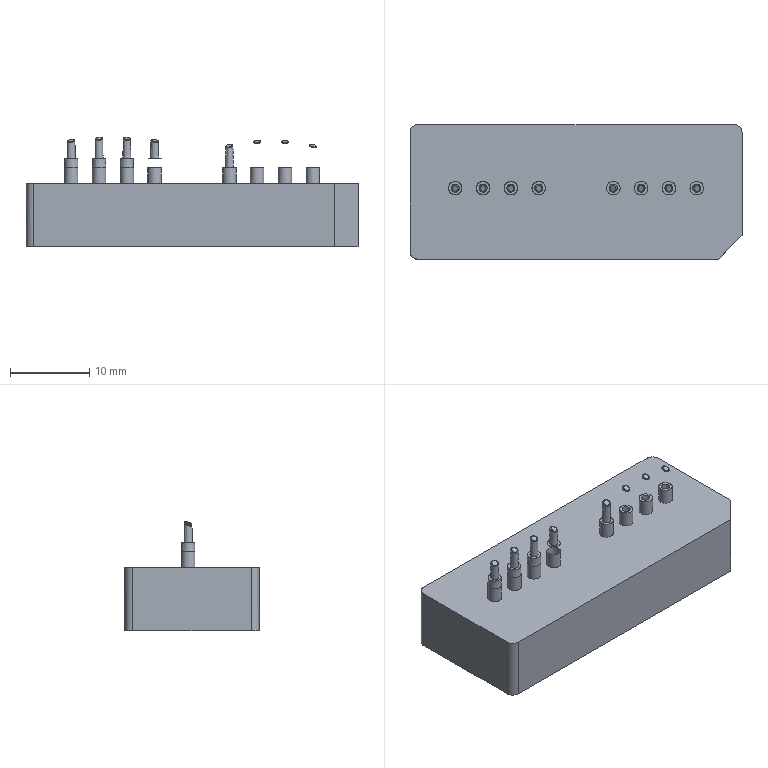NC program | PowerMill | posted by the shop | part box 42 x 17 x 13.856 mm
Lines 4063 to 5561 of 273708:
( TOOL ID   D3C_1_1 )
( TOOL DIA. 3. TIP RAD 0 LENGTH 61.04 )
( Z = -5.95 )
T15 M6
T26
G91 G28 Z0
G0 G90 G54
M08
S18000 M3
X0 Y0 M8
G43 Z9.805 H15
X-10.69 Y-1.921
Z.86
G1 Z-.34 F3000
X-10.681 Y-1.904 F5000
G3 X-10.753 Y-1.67 I-.153 J.081
G1 X-11.82 Y-1.108
X-12.242 Y-1.099
X-12.508 Y-1.055
X-12.664 Y-1.003
X-13.086 Y-.759
X-13.231 Y-.633
X-13.508 Y-.262
X-13.671 Y.211
X-13.709 Y.633
X-13.642 Y1.055
X-13.508 Y1.391
X-13.139 Y1.9
X-12.664 Y2.236
X-12.486 Y2.322
X-12.242 Y2.399
X-11.82 Y2.458
X-11.398 Y2.424
X-11.032 Y2.322
X-10.553 Y2.053
X-10.376 Y1.9
X-10.131 Y1.6
G3 X-9.874 Y1.579 I.135 J.066
G1 X-9.709 Y1.809
X-9.287 Y2.163
X-8.966 Y2.322
X-8.443 Y2.442
X-8.021 Y2.441
X-7.598 Y2.352
X-7.176 Y2.148
X-6.859 Y1.9
X-6.536 Y1.477
X-6.36 Y1.055
X-6.289 Y.633
X-6.328 Y.211
X-6.468 Y-.211
X-6.754 Y-.617
X-7.176 Y-.931
X-7.492 Y-1.055
X-8.021 Y-1.105
X-8.865 Y-1.092
X-9.032 Y-1.055
X-9.287 Y-.951
X-9.725 Y-.633
X-9.87 Y-.434
G3 X-10.04 Y-.384 I-.117 J-.082
G1 X-10.066 Y-.393
X-10.107 Y-.428
X-10.274 Y-.633
X-10.553 Y-.856
X-10.975 Y-1.055
X-11.398 Y-1.117
X-11.82 Y-1.108
X-10.965 Y-2.286 Z-.485
X-10.955 Y-2.27
G3 X-11.003 Y-2.03 I-.144 J.096
G1 X-11.863 Y-1.459
X-12.242 Y-1.412
X-12.664 Y-1.261
X-13.086 Y-.986
X-13.398 Y-.633
X-13.508 Y-.457
X-13.536 Y-.389
X-13.575 Y-.326
G3 X-13.8 Y-.332 I-.11 J-.102
G1 X-13.93 Y-.487
X-14.117 Y-.633
X-14.353 Y-.76
X-14.775 Y-.872
X-15.197 Y-.859
X-15.619 Y-.734
X-16.041 Y-.552
X-16.463 Y-.243
X-16.778 Y.211
X-16.885 Y.602
X-16.886 Y1.055
X-16.763 Y1.477
X-16.463 Y1.905
X-16.041 Y2.224
X-15.822 Y2.322
X-15.619 Y2.381
X-15.197 Y2.418
X-14.775 Y2.358
X-14.353 Y2.194
X-13.951 Y1.9
X-13.67 Y1.531
G3 X-13.432 Y1.531 I.119 J.091
G1 X-13.146 Y1.9
X-12.664 Y2.245
X-12.455 Y2.329
X-12.242 Y2.404
X-11.82 Y2.459
X-11.398 Y2.427
X-11.022 Y2.322
X-10.553 Y2.054
X-10.372 Y1.9
X-10.306 Y1.815
X-10.131 Y1.6
G3 X-9.874 Y1.579 I.135 J.066
G1 X-9.827 Y1.644
X-9.709 Y1.813
X-9.287 Y2.164
X-9.078 Y2.267
X-8.865 Y2.362
X-8.443 Y2.445
X-8.021
X-7.598 Y2.356
X-7.176 Y2.151
X-6.855 Y1.9
X-6.569 Y1.532
G3 X-6.332 Y1.532 I.118 J.092
G1 X-6.043 Y1.9
X-5.91 Y2.018
X-5.488 Y2.271
X-5.066 Y2.39
X-4.643 Y2.417
X-4.221 Y2.334
X-3.799 Y2.128
X-3.522 Y1.9
X-3.377 Y1.721
X-3.238 Y1.477
X-3.119 Y1.055
X-3.126 Y.633
X-3.235 Y.211
X-3.377 Y-.049
X-3.506 Y-.211
X-3.799 Y-.461
X-4.221 Y-.666
X-4.643 Y-.829
X-5.066 Y-.875
X-5.488 Y-.807
X-5.852 Y-.633
X-6.207 Y-.285
G3 X-6.446 Y-.325 I-.105 J-.107
G1 X-6.601 Y-.633
X-6.754 Y-.823
X-7.001 Y-1.055
X-7.176 Y-1.175
X-7.598 Y-1.369
X-8.021 Y-1.454
X-8.443 Y-1.456
X-8.865 Y-1.378
X-9.287 Y-1.185
X-9.486 Y-1.055
X-9.709 Y-.844
X-9.883 Y-.633
G3 X-10.121 Y-.636 I-.118 J-.09
G1 X-10.126 Y-.643
X-10.131 Y-.65
X-10.516 Y-1.055
X-10.975 Y-1.322
X-11.398 Y-1.437
X-11.82 Y-1.464
X-11.863 Y-1.459
X-10.917 Y-2.32 Z-.63
X-10.907 Y-2.304
G3 X-10.962 Y-2.065 I-.147 J.092
G1 X-11.867 Y-1.501
X-12.117 Y-1.477
X-12.664 Y-1.293
X-13.02 Y-1.055
X-13.081 Y-.989
X-13.086 Y-.986
X-13.138 Y-.926
X-13.409 Y-.633
X-13.415 Y-.623
X-13.423 Y-.613
G3 X-13.669 Y-.614 I-.123 J-.082
G1 X-13.682 Y-.633
X-13.93 Y-.885
X-14.182 Y-1.055
X-14.353 Y-1.14
X-14.775 Y-1.252
X-15.197 Y-1.245
X-15.619 Y-1.116
X-16.463 Y-.74
X-16.606 Y-.633
X-16.885 Y-.341
X-16.968 Y-.211
X-17.142 Y.211
X-17.198 Y.633
X-17.139 Y1.055
X-16.971 Y1.477
X-16.885 Y1.626
X-16.661 Y1.9
X-16.463 Y2.07
X-16.041 Y2.313
X-15.619 Y2.43
X-15.197 Y2.462
X-14.775 Y2.4
X-14.353 Y2.237
X-13.93 Y1.94
X-13.638 Y1.559
X-13.62 Y1.544
G3 X-13.406 Y1.563 I.098 J.11
G1 X-13.215 Y1.81
X-13.149 Y1.9
X-12.664 Y2.246
X-12.454 Y2.33
X-12.242 Y2.407
X-11.82 Y2.46
X-11.398 Y2.43
X-11.016 Y2.322
X-10.553 Y2.057
X-10.369 Y1.9
X-10.26 Y1.757
X-10.131 Y1.6
G3 X-9.886 Y1.567 I.134 J.064
G1 X-9.876 Y1.577
X-9.867 Y1.589
X-9.709 Y1.817
X-9.287 Y2.166
X-9.168 Y2.222
X-8.966 Y2.322
X-8.947 Y2.326
X-8.865 Y2.365
X-8.443 Y2.449
X-8.021 Y2.45
X-7.598 Y2.359
X-7.176 Y2.153
X-6.851 Y1.9
X-6.754 Y1.797
X-6.613 Y1.59
G3 X-6.362 Y1.594 I.124 J.085
G1 X-6.332 Y1.642
X-6.111 Y1.9
X-5.91 Y2.071
X-5.467 Y2.322
X-5.066 Y2.432
X-4.643 Y2.46
X-4.221 Y2.399
X-3.981 Y2.322
X-3.799 Y2.232
X-3.377 Y1.933
X-3.024 Y1.477
X-2.857 Y1.055
X-2.806 Y.633
X-2.854 Y.211
X-3.032 Y-.211
X-3.377 Y-.623
X-3.799 Y-.874
X-4.643 Y-1.213
X-5.066 Y-1.261
X-5.488 Y-1.194
X-5.91 Y-1.003
X-6.332 Y-.605
G3 X-6.539 Y-.561 I-.126 J-.082
G1 X-6.569 Y-.589
X-6.586 Y-.608
X-6.599 Y-.63
X-6.601 Y-.633
X-6.628 Y-.667
X-6.754 Y-.843
X-6.978 Y-1.055
X-7.176 Y-1.201
X-7.598 Y-1.402
X-7.879 Y-1.477
X-8.021 Y-1.497
X-8.443 Y-1.493
X-8.865 Y-1.408
X-9.287 Y-1.212
X-9.505 Y-1.055
X-9.709 Y-.862
X-9.882 Y-.644
G3 X-10.131 Y-.666 I-.118 J-.093
G1 X-10.495 Y-1.055
X-10.975 Y-1.351
X-11.398 Y-1.477
X-11.82 Y-1.505
X-11.867 Y-1.501
X-10.955 Y-2.332 Z-.774
X-10.944 Y-2.315
G3 X-10.995 Y-2.076 I-.145 J.095
G1 X-11.868 Y-1.507
X-12.126 Y-1.477
X-12.664 Y-1.296
X-13.025 Y-1.055
X-13.408 Y-.638
G3 X-13.632 Y-.641 I-.111 J-.101
G1 X-13.93 Y-.99
X-14.353 Y-1.281
X-14.775 Y-1.433
X-15.197 Y-1.483
X-15.619 Y-1.443
X-16.041 Y-1.31
X-16.463 Y-1.072
X-16.9 Y-.633
X-17.133 Y-.211
X-17.241 Y.211
X-17.254 Y.633
X-17.179 Y1.055
X-16.991 Y1.477
X-16.885 Y1.648
X-16.667 Y1.9
X-16.463 Y2.072
X-16.041 Y2.315
X-15.619 Y2.434
X-15.197 Y2.465
X-14.775 Y2.401
X-14.525 Y2.322
X-14.353 Y2.24
X-13.93 Y1.941
X-13.639 Y1.562
X-13.623 Y1.547
G3 X-13.406 Y1.564 I.101 J.107
G1 X-13.283 Y1.722
X-13.152 Y1.9
X-12.664 Y2.248
X-12.574 Y2.281
X-12.486 Y2.322
X-12.363 Y2.362
X-12.242 Y2.409
X-11.82 Y2.46
X-11.398 Y2.434
X-11.011 Y2.322
X-10.553 Y2.06
X-10.365 Y1.9
X-10.226 Y1.716
X-10.131 Y1.6
X-10.125 Y1.59
X-10.111 Y1.573
G3 X-9.889 Y1.566 I.114 J.093
G1 X-9.876 Y1.58
X-9.709 Y1.821
X-9.287 Y2.167
X-9.08 Y2.265
X-8.966 Y2.322
X-8.954 Y2.325
X-8.943 Y2.33
X-8.865 Y2.367
X-8.443 Y2.452
X-8.021
X-7.598 Y2.362
X-7.176 Y2.154
X-6.848 Y1.9
X-6.754 Y1.801
X-6.614 Y1.595
G3 X-6.362 Y1.601 I.124 J.085
G1 X-6.332 Y1.65
X-6.113 Y1.9
X-5.91 Y2.073
X-5.474 Y2.322
X-5.066 Y2.434
X-4.643 Y2.466
X-4.221 Y2.401
X-4.007 Y2.329
X-3.799 Y2.241
X-3.377 Y1.942
X-3.005 Y1.477
X-2.82 Y1.055
X-2.743 Y.633
X-2.755 Y.211
X-2.87 Y-.211
X-2.955 Y-.4
X-3.099 Y-.633
X-3.377 Y-.944
X-3.799 Y-1.228
X-4.221 Y-1.398
X-4.656 Y-1.477
X-5.066 Y-1.464
X-5.488 Y-1.346
X-5.91 Y-1.116
X-6.332 Y-.696
X-6.378 Y-.629
X-6.447 Y-.586
X-6.502 Y-.581
X-6.555 Y-.596
X-6.583 Y-.618
X-6.596 Y-.629
X-6.608 Y-.642
X-6.616 Y-.652
X-6.754 Y-.846
X-6.975 Y-1.055
X-7.176 Y-1.204
X-7.598 Y-1.406
X-7.808 Y-1.459
X-8.021 Y-1.499
X-8.443
X-8.865 Y-1.411
X-9.287 Y-1.215
X-9.507 Y-1.055
X-9.709 Y-.865
X-9.882 Y-.648
G3 X-10.122 Y-.657 I-.117 J-.091
G1 X-10.127 Y-.663
X-10.131 Y-.67
X-10.495 Y-1.055
X-10.975 Y-1.353
X-11.398 Y-1.477
X-11.82 Y-1.513
X-11.868 Y-1.507
X-10.969 Y-2.336 Z-.919
X-10.958 Y-2.32
G3 X-11.007 Y-2.08 I-.144 J.096
G1 X-11.868 Y-1.51
X-12.131 Y-1.477
X-12.664 Y-1.299
X-13.028 Y-1.055
X-13.407 Y-.641
G3 X-13.631 Y-.644 I-.111 J-.101
G1 X-13.93 Y-.99
X-14.353 Y-1.289
X-14.775 Y-1.45
X-15.197 Y-1.514
X-15.665 Y-1.477
X-16.041 Y-1.362
X-16.463 Y-1.124
X-16.885 Y-.698
X-17.146 Y-.211
X-17.244 Y.211
X-17.258 Y.633
X-17.18 Y1.055
X-16.995 Y1.477
X-16.885 Y1.655
X-16.667 Y1.9
X-16.463 Y2.074
X-16.041 Y2.317
X-15.619 Y2.438
X-15.197 Y2.468
X-14.775 Y2.402
X-14.519 Y2.322
X-14.353 Y2.243
X-13.93 Y1.943
X-13.64 Y1.565
X-13.594 Y1.525
X-13.535 Y1.509
X-13.463 Y1.52
X-13.405 Y1.565
X-13.346 Y1.641
X-13.156 Y1.9
X-12.664 Y2.25
X-12.519 Y2.306
X-12.486 Y2.322
X-12.438 Y2.337
X-12.242 Y2.412
X-11.82 Y2.461
X-11.398 Y2.437
X-11.005 Y2.322
X-10.553 Y2.063
X-10.362 Y1.9
X-10.131 Y1.613
G3 X-9.871 Y1.591 I.136 J.066
G1 X-9.709 Y1.824
X-9.287 Y2.168
X-8.865 Y2.37
X-8.443 Y2.454
X-8.021 Y2.455
X-7.598 Y2.364
X-7.176 Y2.155
X-6.844 Y1.9
X-6.754 Y1.804
X-6.613 Y1.599
G3 X-6.361 Y1.606 I.124 J.085
G1 X-6.332 Y1.654
X-6.116 Y1.9
X-5.91 Y2.074
X-5.488 Y2.319
X-5.066 Y2.435
X-4.643 Y2.47
X-4.221 Y2.403
X-4.009 Y2.328
X-3.799 Y2.244
X-3.377 Y1.944
X-3.002 Y1.477
X-2.819 Y1.055
X-2.737 Y.633
X-2.753 Y.211
X-2.856 Y-.211
X-3.07 Y-.633
X-3.377 Y-.988
X-3.799 Y-1.285
X-4.337 Y-1.477
X-4.643 Y-1.514
X-5.066 Y-1.485
X-5.488 Y-1.364
X-5.696 Y-1.235
X-5.91 Y-1.116
X-5.949 Y-1.081
X-5.995 Y-1.055
X-6.332 Y-.701
X-6.373 Y-.638
X-6.434 Y-.594
G3 X-6.609 Y-.647 I-.053 J-.14
G1 X-6.754 Y-.849
X-6.973 Y-1.055
X-7.176 Y-1.207
X-7.598 Y-1.409
X-7.809 Y-1.458
X-8.021 Y-1.501
X-8.443 Y-1.503
X-8.865 Y-1.413
X-9.287 Y-1.218
X-9.509 Y-1.055
X-9.709 Y-.868
X-9.882 Y-.652
G3 X-10.131 Y-.674 I-.117 J-.094
G1 X-10.494 Y-1.055
X-10.975 Y-1.356
X-11.398 Y-1.477
X-11.82 Y-1.515
X-11.868 Y-1.51
X-10.98 Y-2.341 Z-1.064
X-10.969 Y-2.325
G3 X-11.017 Y-2.084 I-.144 J.097
G1 X-11.868 Y-1.512
X-12.136 Y-1.477
X-12.664 Y-1.302
X-13.03 Y-1.055
X-13.408 Y-.644
G3 X-13.631 Y-.647 I-.11 J-.101
G1 X-13.93 Y-.99
X-14.353 Y-1.292
X-14.775 Y-1.45
X-15.197 Y-1.517
X-15.619 Y-1.487
X-15.65 Y-1.479
X-15.665 Y-1.477
X-15.812 Y-1.432
X-16.041 Y-1.367
X-16.463 Y-1.126
X-16.885 Y-.7
X-17.148 Y-.211
X-17.248 Y.211
X-17.262 Y.633
X-17.183 Y1.055
X-17. Y1.477
X-16.885 Y1.66
X-16.667 Y1.9
X-16.463 Y2.076
X-16.041 Y2.32
X-15.619 Y2.44
X-15.197 Y2.471
X-14.775 Y2.403
X-14.512 Y2.322
X-14.353 Y2.246
X-13.93 Y1.946
X-13.642 Y1.568
G3 X-13.402 Y1.571 I.119 J.091
G1 X-13.159 Y1.9
X-12.664 Y2.252
X-12.496 Y2.317
X-12.486 Y2.322
X-12.473 Y2.326
X-12.242 Y2.415
X-11.82 Y2.462
X-11.398 Y2.44
X-10.999 Y2.322
X-10.553 Y2.067
X-10.358 Y1.9
X-10.131 Y1.617
G3 X-9.872 Y1.596 I.136 J.066
G1 X-9.709 Y1.828
X-9.287 Y2.169
X-8.865 Y2.373
X-8.443 Y2.457
X-8.021
X-7.598 Y2.367
X-7.176 Y2.158
X-6.841 Y1.9
X-6.754 Y1.808
X-6.613 Y1.603
G3 X-6.361 Y1.611 I.124 J.085
G1 X-6.332 Y1.659
X-6.12 Y1.9
X-5.91 Y2.076
X-5.488 Y2.322
X-5.066 Y2.437
X-4.643 Y2.472
X-4.221 Y2.405
X-4.113 Y2.364
X-3.981 Y2.322
X-3.892 Y2.28
X-3.799 Y2.247
X-3.377 Y1.946
X-2.999 Y1.477
X-2.816 Y1.055
X-2.734 Y.633
X-2.75 Y.211
X-2.851 Y-.211
X-3.07 Y-.633
X-3.377 Y-.993
X-3.799 Y-1.289
X-4.334 Y-1.477
X-4.643 Y-1.517
X-5.066 Y-1.485
X-5.488 Y-1.367
X-5.804 Y-1.174
X-5.91 Y-1.116
X-5.928 Y-1.098
X-5.998 Y-1.055
X-6.332 Y-.705
X-6.373 Y-.642
X-6.433 Y-.598
X-6.518 Y-.591
X-6.592 Y-.633
X-6.609 Y-.651
X-6.754 Y-.852
X-6.97 Y-1.055
X-7.176 Y-1.21
X-7.598 Y-1.411
X-7.788 Y-1.453
X-7.858 Y-1.473
X-7.93 Y-1.484
X-8.021 Y-1.504
X-8.443 Y-1.506
X-8.865 Y-1.416
X-9.287 Y-1.222
X-9.511 Y-1.055
X-9.709 Y-.872
X-9.882 Y-.656
G3 X-10.131 Y-.679 I-.117 J-.094
G1 X-10.491 Y-1.055
X-10.975 Y-1.359
X-11.398 Y-1.477
X-11.82 Y-1.518
X-11.868 Y-1.512
X-10.989 Y-2.345 Z-1.209
X-10.978 Y-2.329
G3 X-11.024 Y-2.088 I-.143 J.097
G1 X-11.869 Y-1.514
X-12.141 Y-1.477
X-12.664 Y-1.305
X-13.032 Y-1.055
X-13.408 Y-.647
G3 X-13.631 Y-.65 I-.11 J-.102
G1 X-13.93 Y-.99
X-14.353 Y-1.295
X-14.775 Y-1.451
X-15.197 Y-1.519
X-15.619 Y-1.491
X-16.041 Y-1.369
X-16.463 Y-1.128
X-16.885 Y-.704
X-17.151 Y-.211
X-17.251 Y.211
X-17.265 Y.633
X-17.186 Y1.055
X-17.003 Y1.477
X-16.885 Y1.664
X-16.669 Y1.9
X-16.463 Y2.078
X-16.041 Y2.322
X-15.619 Y2.442
X-15.197 Y2.473
X-14.775 Y2.405
X-14.506 Y2.322
X-14.353 Y2.249
X-13.93 Y1.949
X-13.635 Y1.577
G3 X-13.397 Y1.582 I.117 J.093
G1 X-13.163 Y1.9
X-12.664 Y2.254
X-12.242 Y2.417
X-11.82 Y2.463
X-11.398 Y2.442
X-11.068 Y2.342
X-10.999 Y2.322
X-10.993 Y2.32
X-10.987 Y2.318
X-10.975 Y2.314
X-10.553 Y2.069
X-10.355 Y1.9
X-10.131 Y1.62
G3 X-9.872 Y1.599 I.136 J.067
G1 X-9.709 Y1.832
X-9.287 Y2.17
X-8.865 Y2.375
X-8.443 Y2.459
X-8.021 Y2.46
X-7.598 Y2.369
X-7.176 Y2.161
X-6.837 Y1.9
X-6.826 Y1.884
X-6.754 Y1.808
X-6.613 Y1.603
X-6.549 Y1.551
X-6.467 Y1.54
X-6.44 Y1.549
X-6.404 Y1.569
X-6.374 Y1.598
X-6.365 Y1.608
X-6.332 Y1.663
X-6.124 Y1.9
X-5.91 Y2.077
X-5.494 Y2.322
X-5.066 Y2.439
X-4.643 Y2.475
X-4.221 Y2.406
X-4.072 Y2.351
X-4.007 Y2.332
X-3.945 Y2.304
X-3.799 Y2.25
X-3.377 Y1.948
X-2.996 Y1.477
X-2.813 Y1.055
X-2.732 Y.633
X-2.748 Y.211
X-2.848 Y-.211
X-3.067 Y-.633
X-3.377 Y-.996
X-3.799 Y-1.293
X-4.332 Y-1.477
X-4.643 Y-1.519
X-5.066 Y-1.485
X-5.488 Y-1.37
X-5.832 Y-1.158
X-5.91 Y-1.116
X-5.924 Y-1.102
X-6. Y-1.055
X-6.332 Y-.709
X-6.373 Y-.645
X-6.434 Y-.6
G3 X-6.611 Y-.653 I-.054 J-.14
G1 X-6.754 Y-.855
X-6.787 Y-.883
X-6.97 Y-1.055
X-7.146 Y-1.187
X-7.176 Y-1.213
X-7.598 Y-1.413
X-7.834 Y-1.465
X-7.879 Y-1.477
X-7.903 Y-1.481
X-8.021 Y-1.507
X-8.443 Y-1.508
X-8.865 Y-1.418
X-9.287 Y-1.224
X-9.32 Y-1.197
X-9.511 Y-1.055
X-9.678 Y-.901
X-9.709 Y-.875
X-9.882 Y-.66
G3 X-10.131 Y-.683 I-.117 J-.094
G1 X-10.489 Y-1.055
X-10.975 Y-1.361
X-11.395 Y-1.477
X-11.82 Y-1.521
X-11.869 Y-1.514
G0 Z3.57
G1 X5.805 Y-.192 F10000
G0 Z.57
G1 Z-.63 F3000
X5.822 Y-.202 F5000
G3 X6.058 Y-.137 I.086 J.151
G1 X6.496 Y.633
X6.519 Y1.055
X6.667 Y1.477
X6.754 Y1.625
X6.983 Y1.9
X7.176 Y2.068
X7.598 Y2.305
X8.021 Y2.408
X8.443 Y2.409
X8.865 Y2.317
X9.287 Y2.108
X9.542 Y1.9
X9.709 Y1.713
X9.858 Y1.477
X9.863 Y1.468
X9.868 Y1.458
G3 X10.141 Y1.477 I.132 J.069
G1 X10.463 Y1.9
X10.553 Y1.985
X10.975 Y2.257
X11.135 Y2.322
X11.398 Y2.383
X11.82 Y2.423
X12.242 Y2.357
X12.664 Y2.172
X13.017 Y1.9
X13.335 Y1.477
X13.483 Y1.055
X13.504 Y.633
X13.401 Y.211
X13.158 Y-.211
X13.086 Y-.296
X12.64 Y-.633
X12.242 Y-.763
X11.82 Y-.832
X11.398 Y-.864
X10.975 Y-.778
X10.674 Y-.633
X10.553 Y-.548
X10.219 Y-.211
X10.131 Y-.074
G3 X9.858 Y-.061 I-.139 J-.056
G1 X9.781 Y-.211
X9.709 Y-.304
X9.327 Y-.633
X8.865 Y-.828
X8.443 Y-.865
X7.598 Y-.724
X7.364 Y-.633
X7.176 Y-.522
X6.842 Y-.211
X6.596 Y.211
X6.496 Y.633
X5.482 Y-.17 Z-.774
X5.498 Y-.181
G3 X5.739 Y-.14 I.1 J.141
G1 X6.309 Y.662
X6.37 Y1.055
X6.546 Y1.477
X6.754 Y1.765
X6.88 Y1.9
X7.176 Y2.133
X7.549 Y2.322
X8.021 Y2.435
X8.443 Y2.431
X8.865 Y2.341
X9.287 Y2.145
X9.605 Y1.9
X9.709 Y1.789
X9.867 Y1.559
G3 X10.12 Y1.568 I.124 J.085
G1 X10.131 Y1.587
X10.396 Y1.9
X10.553 Y2.034
X10.975 Y2.285
X11.398 Y2.411
X11.82 Y2.441
X12.242 Y2.384
X12.452 Y2.322
X12.664 Y2.223
X13.086 Y1.932
X13.453 Y1.477
X13.631 Y1.055
X13.695 Y.633
X13.667 Y.211
X13.508 Y-.226
X13.208 Y-.633
X13.086 Y-.746
X12.664 Y-.996
X12.473 Y-1.055
X12.242 Y-1.098
X11.398 Y-1.206
X10.975 Y-1.134
X10.779 Y-1.055
X10.553 Y-.925
X10.217 Y-.633
X10.121 Y-.493
G3 X9.869 Y-.498 I-.124 J-.085
G1 X9.709 Y-.717
X9.287 Y-1.02
X8.865 Y-1.174
X8.443 Y-1.2
X7.523 Y-1.055
X7.176 Y-.921
X6.786 Y-.633
X6.478 Y-.211
X6.333 Y.211
X6.304 Y.633
X6.309 Y.662
X5.405 Y-.206 Z-.919
X5.421 Y-.217
G3 X5.663 Y-.179 I.102 J.14
G1 X6.281 Y.667
X6.332 Y.968
X6.541 Y1.477
X6.596 Y1.547
X6.754 Y1.765
X6.85 Y1.867
X6.854 Y1.872
X6.875 Y1.9
X7.176 Y2.137
X7.543 Y2.322
X8.021 Y2.438
X8.443 Y2.432
X8.865 Y2.346
X9.287 Y2.149
X9.608 Y1.9
X9.709 Y1.795
X9.867 Y1.561
G3 X10.121 Y1.569 I.124 J.084
G1 X10.131 Y1.587
X10.392 Y1.9
X10.553 Y2.036
X10.975 Y2.288
X11.398 Y2.413
X11.82 Y2.445
X12.242 Y2.387
X12.457 Y2.322
X12.664 Y2.226
X13.086 Y1.937
X13.458 Y1.477
X13.643 Y1.055
X13.725 Y.633
X13.711 Y.211
X13.606 Y-.211
X13.508 Y-.426
X13.376 Y-.633
X13.086 Y-.958
X12.97 Y-1.055
X12.664 Y-1.244
X12.242 Y-1.393
X11.82 Y-1.457
X11.398 Y-1.436
X10.975 Y-1.314
X10.553 Y-1.071
X10.129 Y-.633
G3 X9.872 Y-.61 I-.136 J-.065
G1 X9.709 Y-.834
X9.47 Y-1.055
X9.287 Y-1.181
X8.865 Y-1.372
X8.443 Y-1.453
X8.021 Y-1.441
X7.598 Y-1.348
X7.176 Y-1.157
X7.029 Y-1.055
X6.754 Y-.804
X6.62 Y-.633
X6.398 Y-.211
X6.287 Y.211
X6.275 Y.633
X6.281 Y.667
X4.64 Y3.219 Z-1.064
X4.636 Y3.201
G3 X4.766 Y2.993 I.169 J-.038
G1 X7.631 Y2.345
X8.021 Y2.44
X8.443 Y2.433
X8.865 Y2.352
X9.287 Y2.152
X9.33 Y2.116
X9.608 Y1.9
X9.686 Y1.819
X9.709 Y1.8
X9.867 Y1.564
G3 X10.131 Y1.589 I.125 J.085
G1 X10.388 Y1.9
X10.553 Y2.039
X10.975 Y2.291
X11.398 Y2.415
X11.82 Y2.448
X12.242 Y2.39
X12.463 Y2.322
X12.664 Y2.227
X13.086 Y1.94
X13.454 Y1.486
G3 X13.689 Y1.488 I.117 J.094
G1 X14.01 Y1.9
X14.353 Y2.143
X14.775 Y2.315
X15.197 Y2.379
X15.619 Y2.324
X16.041 Y2.147
X16.354 Y1.9
X16.463 Y1.775
X16.64 Y1.477
X16.766 Y1.055
X16.761 Y.633
X16.635 Y.211
X16.463 Y-.091
X16.363 Y-.211
X16.041 Y-.488
X15.619 Y-.697
X15.197 Y-.803
X14.775 Y-.787
X14.353 Y-.664
X13.93 Y-.366
X13.816 Y-.243
X13.795 Y-.227
G3 X13.573 Y-.284 I-.089 J-.117
G1 X13.544 Y-.346
X13.508 Y-.438
X13.391 Y-.633
X13.086 Y-.982
X12.664 Y-1.271
X12.242 Y-1.436
X12.041 Y-1.477
X11.82 Y-1.493
X11.491 Y-1.477
X10.975 Y-1.334
X10.553 Y-1.083
X10.344 Y-.855
X10.129 Y-.633
G3 X9.89 Y-.614 I-.126 J-.075
G1 X9.882 Y-.624
X9.878 Y-.628
X9.875 Y-.633
X9.709 Y-.839
X9.486 Y-1.055
X9.287 Y-1.197
X8.865 Y-1.395
X8.515 Y-1.477
X7.958
X7.598 Y-1.387
X7.176 Y-1.186
X6.997 Y-1.055
X6.754 Y-.817
X6.611 Y-.633
X6.417 Y-.256
G3 X6.176 Y-.22 I-.133 J-.069
G1 X5.91 Y-.493
X5.68 Y-.633
X5.488 Y-.713
X5.066 Y-.796
X4.643 Y-.771
X4.245 Y-.633
X3.799 Y-.363
X3.645 Y-.211
X3.371 Y.211
X3.245 Y.633
X3.244 Y1.055
X3.364 Y1.477
X3.65 Y1.9
X3.799 Y2.026
X4.221 Y2.27
X4.395 Y2.322
X4.643 Y2.357
X5.066 Y2.346
X5.488 Y2.222
X5.91 Y1.955
X6.307 Y1.477
G3 X6.54 Y1.48 I.115 J.096
G1 X6.702 Y1.692
X6.871 Y1.9
X7.176 Y2.141
X7.538 Y2.322
X7.631 Y2.345
X4.616 Y3.346 Z-1.209
X4.611 Y3.327
G3 X4.743 Y3.12 I.169 J-.038
G1 X7.899 Y2.413
X8.021 Y2.443
X8.443 Y2.434
X8.865 Y2.355
X9.287 Y2.154
X9.502 Y1.984
X9.709 Y1.803
X9.866 Y1.567
G3 X10.121 Y1.575 I.125 J.083
G1 X10.131 Y1.593
X10.384 Y1.9
X10.553 Y2.04
X10.975 Y2.293
X11.398 Y2.417
X11.82 Y2.451
X12.242 Y2.393
X12.468 Y2.322
X12.664 Y2.23
X12.9 Y2.068
X13.132 Y1.9
X13.266 Y1.719
X13.407 Y1.544
G3 X13.621 Y1.528 I.114 J.093
G1 X13.638 Y1.544
X13.904 Y1.9
X14.353 Y2.223
X14.563 Y2.322
X14.775 Y2.388
X15.197 Y2.448
X15.619 Y2.425
X15.976 Y2.322
X16.463 Y2.039
X16.623 Y1.9
X16.885 Y1.55
X17.075 Y1.055
X17.112 Y.633
X17.029 Y.211
X16.811 Y-.211
X16.463 Y-.562
X15.498 Y-1.055
X15.197 Y-1.137
X14.775 Y-1.148
X14.353 Y-1.051
X13.93 Y-.805
X13.754 Y-.633
X13.69 Y-.544
G3 X13.438 Y-.557 I-.122 J-.087
G1 X13.394 Y-.633
X13.086 Y-.986
X12.664 Y-1.277
X12.242 Y-1.439
X12.058 Y-1.477
X11.82 Y-1.497
X11.491 Y-1.477
X10.975 Y-1.338
X10.553 Y-1.086
X10.295 Y-.804
X10.129 Y-.633
G3 X9.894 Y-.614 I-.125 J-.078
G1 X9.877 Y-.633
X9.709 Y-.843
X9.489 Y-1.055
X9.287 Y-1.199
X8.865 Y-1.397
X8.515 Y-1.477
X8.021 Y-1.485
X7.99 Y-1.478
X7.958 Y-1.477
X7.604 Y-1.388
X7.598 Y-1.387
X7.176 Y-1.189
X6.992 Y-1.055
X6.754 Y-.822
X6.607 Y-.633
X6.574 Y-.571
X6.53 Y-.515
G3 X6.31 Y-.54 I-.099 J-.113
G1 X6.243 Y-.633
X5.91 Y-.914
X5.488 Y-1.097
X5.066 Y-1.154
X4.643 Y-1.097
X4.519 Y-1.055
X3.653 Y-.633
X3.377 Y-.423
X3.196 Y-.211
X2.976 Y.211
X2.892 Y.633
X2.928 Y1.055
X3.08 Y1.477
X3.381 Y1.9
X3.799 Y2.215
X4.221 Y2.386
X4.643 Y2.452
X5.066 Y2.423
X5.436 Y2.322
X5.91 Y2.06
X6.094 Y1.9
X6.332 Y1.627
X6.373 Y1.564
X6.433 Y1.52
X6.527 Y1.515
X6.606 Y1.567
X6.734 Y1.735
X6.868 Y1.9
X7.176 Y2.143
X7.533 Y2.322
X7.899 Y2.413
X4.579 Y3.347 Z-1.354
X4.575 Y3.329
G3 X4.707 Y3.122 I.169 J-.037
G1 X7.898 Y2.415
X8.021 Y2.445
X8.443 Y2.436
X8.865 Y2.357
X9.287 Y2.156
X9.5 Y1.984
X9.709 Y1.807
X9.866 Y1.571
G3 X10.121 Y1.579 I.125 J.083
G1 X10.131 Y1.597
X10.381 Y1.9
X10.553 Y2.042
X10.975 Y2.296
X11.398 Y2.419
X11.82 Y2.453
X12.242 Y2.395
X12.279 Y2.381
X12.468 Y2.322
X12.631 Y2.245
X12.664 Y2.232
X13.086 Y1.946
X13.105 Y1.92
X13.132 Y1.9
X13.266 Y1.719
X13.406 Y1.545
G3 X13.62 Y1.529 I.114 J.093
G1 X13.637 Y1.545
X13.899 Y1.9
X14.353 Y2.223
X14.354 Y2.224
X14.563 Y2.322
X14.734 Y2.375
X14.775 Y2.392
X15.197 Y2.451
X15.619 Y2.427
X15.997 Y2.322
X16.463 Y2.063
X16.648 Y1.9
X16.885 Y1.63
X16.985 Y1.477
X17.164 Y1.055
X17.231 Y.633
X17.206 Y.211
X17.064 Y-.211
X16.773 Y-.633
X16.463 Y-.893
X15.619 Y-1.302
X15.197 Y-1.388
X14.775 Y-1.365
X14.353 Y-1.234
X14.058 Y-1.055
X13.93 Y-.951
X13.643 Y-.633
G3 X13.397 Y-.633 I-.123 J-.086
G1 X13.086 Y-.989
X12.664 Y-1.281
X12.242 Y-1.441
X12.075 Y-1.477
X11.82 Y-1.502
X11.482 Y-1.477
X10.975 Y-1.34
X10.553 Y-1.089
X10.232 Y-.739
X10.129 Y-.633
X10.114 Y-.614
X10.096 Y-.598
X10.073 Y-.581
G3 X9.88 Y-.633 I-.067 J-.134
G1 X9.709 Y-.847
X9.492 Y-1.055
X9.287 Y-1.202
X8.865 Y-1.4
X8.519 Y-1.477
X8.021 Y-1.489
X7.987 Y-1.481
X7.972 Y-1.479
X7.958 Y-1.477
X7.727 Y-1.419
X7.598 Y-1.388
X7.176 Y-1.192
X6.988 Y-1.055
X6.754 Y-.824
X6.603 Y-.633
G3 X6.353 Y-.637 I-.124 J-.084
G1 X6.332 Y-.669
X5.94 Y-1.055
X5.488 Y-1.298
X5.066 Y-1.38
X4.643 Y-1.366
X4.221 Y-1.231
X3.799 Y-1.024
X3.377 Y-.769
X3.232 Y-.633
X2.955 Y-.242
X2.796 Y.211
X2.765 Y.633
X2.836 Y1.055
X3.016 Y1.477
X3.346 Y1.9
X3.799 Y2.223
X4.003 Y2.322
X4.221 Y2.39
X4.643 Y2.453
X5.066 Y2.426
X5.439 Y2.322
X5.91 Y2.06
X6.102 Y1.9
X6.332 Y1.629
X6.372 Y1.567
X6.432 Y1.524
X6.527 Y1.518
X6.605 Y1.57
X6.701 Y1.692
X6.754 Y1.765
X6.784 Y1.797
X6.865 Y1.9
X7.176 Y2.146
X7.527 Y2.322
X7.898 Y2.415
G0 Z2.846
G1 X-2.04 Y1.895 F10000
G0 Z-.154
G1 Z-1.354 F3000
X-2.133 Y1.726 F5000
X-2.73 Y.633
X-2.745 Y.211
X-2.845 Y-.211
X-3.064 Y-.633
X-3.377 Y-1.
X-3.799 Y-1.296
X-4.33 Y-1.477
X-4.643 Y-1.522
X-5.066 Y-1.485
X-5.488 Y-1.372
X-5.861 Y-1.142
X-5.91 Y-1.116
X-5.919 Y-1.107
X-6.003 Y-1.055
X-6.332 Y-.713
X-6.373 Y-.649
X-6.434 Y-.605
G3 X-6.61 Y-.657 I-.054 J-.14
G1 X-6.754 Y-.859
X-6.961 Y-1.043
X-7.176 Y-1.216
X-7.598 Y-1.415
X-8.021 Y-1.509
X-8.443 Y-1.511
X-8.865 Y-1.421
X-9.287 Y-1.227
X-9.503 Y-1.058
X-9.709 Y-.878
X-9.882 Y-.664
G3 X-10.119 Y-.671 I-.116 J-.092
G1 X-10.126 Y-.679
X-10.131 Y-.687
X-10.487 Y-1.055
X-10.975 Y-1.364
X-11.385 Y-1.477
X-11.82 Y-1.523
X-12.145 Y-1.477
X-12.664 Y-1.308
X-13.033 Y-1.055
X-13.408 Y-.65
G3 X-13.631 Y-.653 I-.11 J-.102
G1 X-13.93 Y-.992
X-14.353 Y-1.298
X-14.775 Y-1.452
X-15.197 Y-1.522
X-15.619 Y-1.492
X-16.041 Y-1.372
X-16.463 Y-1.13
X-16.885 Y-.708
X-17.154 Y-.211
X-17.254 Y.211
X-17.268 Y.633
X-17.188 Y1.055
X-17.006 Y1.477
X-16.885 Y1.668
X-16.673 Y1.9
X-16.463 Y2.08
X-16.048 Y2.322
X-15.619 Y2.444
X-15.197 Y2.476
X-14.775 Y2.406
X-14.743 Y2.395
X-14.506 Y2.322
X-14.38 Y2.262
X-14.353 Y2.252
X-13.93 Y1.952
X-13.636 Y1.582
G3 X-13.401 Y1.581 I.117 J.093
G1 X-13.344 Y1.652
X-13.163 Y1.9
X-13.119 Y1.932
X-13.086 Y1.976
X-12.664 Y2.255
X-12.242 Y2.42
X-11.82 Y2.466
X-11.398 Y2.445
X-10.988 Y2.322
X-10.553 Y2.072
X-10.351 Y1.9
X-10.131 Y1.624
G3 X-9.872 Y1.603 I.136 J.067
G1 X-9.709 Y1.835
X-9.287 Y2.172
X-8.865 Y2.378
X-8.443 Y2.462
X-8.021
X-7.598 Y2.372
X-7.176 Y2.164
X-6.834 Y1.9
X-6.81 Y1.867
X-6.754 Y1.808
X-6.613 Y1.603
X-6.606 Y1.594
X-6.56 Y1.558
X-6.504 Y1.543
X-6.424 Y1.557
X-6.365 Y1.613
X-6.332 Y1.667
X-6.127 Y1.9
X-5.91 Y2.079
X-5.5 Y2.322
X-5.066 Y2.441
X-4.643 Y2.477
X-4.221 Y2.408
X-4.024 Y2.335
X-3.981 Y2.322
X-3.966 Y2.314
X-3.799 Y2.253
X-3.377 Y1.95
X-2.994 Y1.477
X-2.811 Y1.055
X-2.73 Y.633
X1.71 Y-.716 Z-1.499
X1.828 Y-.564
X2.75 Y.633
X2.832 Y1.055
X2.955 Y1.372
X2.991 Y1.421
X3.016 Y1.477
X3.289 Y1.827
X3.342 Y1.9
X3.799 Y2.225
X3.997 Y2.322
X4.221 Y2.395
X4.643 Y2.455
X5.066 Y2.429
X5.445 Y2.322
X5.91 Y2.062
X6.106 Y1.9
X6.251 Y1.726
X6.391 Y1.548
G3 X6.605 Y1.57 I.097 J.115
G1 X6.701 Y1.692
X6.754 Y1.765
X6.784 Y1.797
X6.801 Y1.819
X6.862 Y1.9
X7.176 Y2.149
X7.522 Y2.322
X8.021 Y2.448
X8.443 Y2.438
X8.865 Y2.36
X9.287 Y2.158
X9.484 Y1.996
X9.608 Y1.899
X9.635 Y1.871
X9.709 Y1.811
X9.867 Y1.575
G3 X10.121 Y1.583 I.125 J.083
G1 X10.131 Y1.601
X10.377 Y1.9
X10.553 Y2.045
X10.975 Y2.299
X11.398 Y2.422
X11.82 Y2.456
X12.242 Y2.398
X12.455 Y2.323
X12.664 Y2.235
X13.086 Y1.95
X13.103 Y1.928
X13.116 Y1.913
X13.132 Y1.9
X13.261 Y1.725
X13.397 Y1.556
G3 X13.613 Y1.541 I.114 J.093
G1 X13.628 Y1.556
X13.895 Y1.9
X14.353 Y2.223
X14.554 Y2.322
X14.775 Y2.395
X15.197 Y2.453
X15.619 Y2.43
X16.002 Y2.322
X16.463 Y2.066
X16.653 Y1.9
X16.885 Y1.633
X16.986 Y1.477
X17.17 Y1.055
X17.249 Y.633
X17.24 Y.211
X17.136 Y-.211
X16.915 Y-.633
X16.517 Y-1.055
X16.041 Y-1.34
X15.547 Y-1.477
X15.197 Y-1.5
X14.95 Y-1.477
X14.775 Y-1.435
X14.353 Y-1.277
X14.021 Y-1.055
X13.634 Y-.633
G3 X13.4 Y-.633 I-.117 J-.094
G1 X13.086 Y-.992
X12.664 Y-1.283
X12.242 Y-1.444
X12.032 Y-1.482
X11.82 Y-1.504
X11.468 Y-1.477
X10.975 Y-1.343
X10.553 Y-1.092
X10.169 Y-.674
X10.129 Y-.633
X10.117 Y-.619
X10.102 Y-.606
G3 X9.884 Y-.633 I-.097 J-.109
G1 X9.709 Y-.851
X9.495 Y-1.055
X9.287 Y-1.205
X8.865 Y-1.403
X8.531 Y-1.477
X8.021 Y-1.492
X7.959 Y-1.477
X7.958
X7.938 Y-1.472
X7.598 Y-1.391
X7.176 Y-1.195
X6.984 Y-1.055
X6.754 Y-.827
X6.6 Y-.633
G3 X6.354 Y-.647 I-.119 J-.092
G1 X6.332 Y-.682
X5.981 Y-1.055
X5.488 Y-1.351
X5.046 Y-1.477
X4.643 Y-1.497
X4.221 Y-1.429